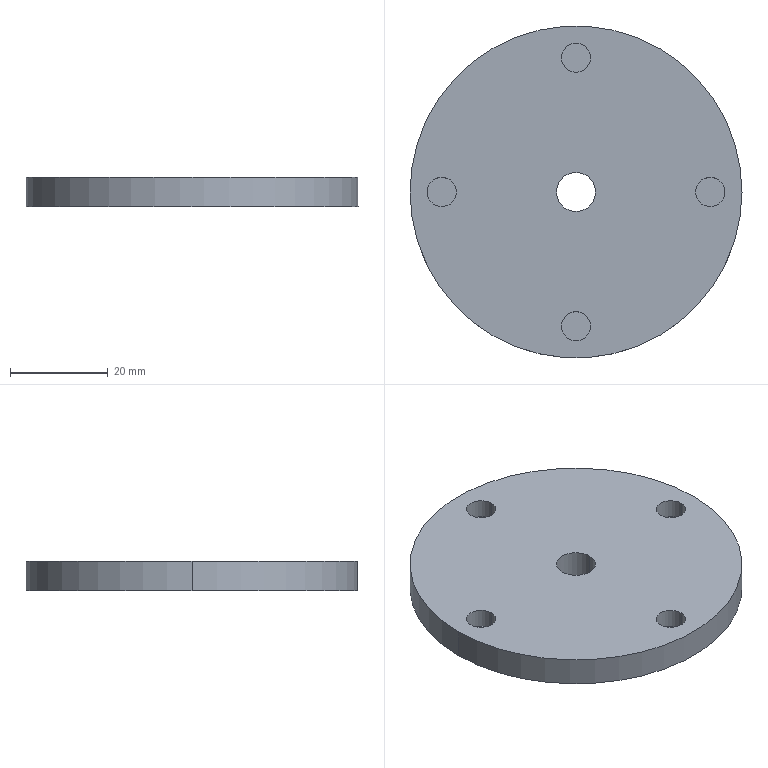Part | SolidWorks | features ICE 2, Extrusion 1 | 1 solid | 18 faces | box 68 x 68 x 6 mm | volume 21036 mm3 | cylinder 12 | plane 6 | commonest cylinder face diameters 6 x8 8 x2 68 x2
STEP:
#1=CARTESIAN_POINT('',(-4.,0.,0.));
#2=VERTEX_POINT('',#1);
#3=CARTESIAN_POINT('',(4.,0.,0.));
#4=VERTEX_POINT('',#3);
#5=CARTESIAN_POINT('',(0.,0.,0.));
#6=DIRECTION('',(0.,0.,1.));
#7=DIRECTION('',(1.,0.,0.));
#8=AXIS2_PLACEMENT_3D('',#5,#6,#7);
#9=CIRCLE('',#8,4.);
#10=EDGE_CURVE('',#2,#4,#9,.T.);
#11=ORIENTED_EDGE('',*,*,#10,.F.);
#12=CARTESIAN_POINT('',(-4.,0.,6.));
#13=VERTEX_POINT('',#12);
#14=CARTESIAN_POINT('',(-4.,0.,0.));
#15=DIRECTION('',(0.,0.,1.));
#16=VECTOR('',#15,1000.);
#17=LINE('',#14,#16);
#18=EDGE_CURVE('',#2,#13,#17,.T.);
#19=ORIENTED_EDGE('',*,*,#18,.T.);
#20=CARTESIAN_POINT('',(4.,0.,6.));
#21=VERTEX_POINT('',#20);
#22=CARTESIAN_POINT('',(0.,0.,6.));
#23=DIRECTION('',(0.,0.,1.));
#24=DIRECTION('',(1.,0.,0.));
#25=AXIS2_PLACEMENT_3D('',#22,#23,#24);
#26=CIRCLE('',#25,4.);
#27=EDGE_CURVE('',#13,#21,#26,.T.);
#28=ORIENTED_EDGE('',*,*,#27,.T.);
#29=CARTESIAN_POINT('',(4.,0.,0.));
#30=DIRECTION('',(0.,0.,1.));
#31=VECTOR('',#30,1000.);
#32=LINE('',#29,#31);
#33=EDGE_CURVE('',#4,#21,#32,.T.);
#34=ORIENTED_EDGE('',*,*,#33,.F.);
#35=EDGE_LOOP('',(#11,#19,#28,#34));
#36=FACE_OUTER_BOUND('',#35,.T.);
#37=CARTESIAN_POINT('',(0.,0.,0.));
#38=DIRECTION('',(0.,0.,1.));
#39=DIRECTION('',(1.,0.,0.));
#40=AXIS2_PLACEMENT_3D('',#37,#38,#39);
#41=CYLINDRICAL_SURFACE('',#40,4.);
#42=ADVANCED_FACE('',(#36),#41,.F.);
#43=CARTESIAN_POINT('',(-3.,27.5,2.));
#44=VERTEX_POINT('',#43);
#45=CARTESIAN_POINT('',(3.,27.5,2.));
#46=VERTEX_POINT('',#45);
#47=CARTESIAN_POINT('',(0.,27.5,2.));
#48=DIRECTION('',(0.,0.,1.));
#49=DIRECTION('',(1.,0.,0.));
#50=AXIS2_PLACEMENT_3D('',#47,#48,#49);
#51=CIRCLE('',#50,3.);
#52=EDGE_CURVE('',#44,#46,#51,.T.);
#53=ORIENTED_EDGE('',*,*,#52,.F.);
#54=CARTESIAN_POINT('',(-3.,27.5,6.));
#55=VERTEX_POINT('',#54);
#56=CARTESIAN_POINT('',(-3.,27.5,2.));
#57=DIRECTION('',(0.,0.,1.));
#58=VECTOR('',#57,1000.);
#59=LINE('',#56,#58);
#60=EDGE_CURVE('',#44,#55,#59,.T.);
#61=ORIENTED_EDGE('',*,*,#60,.T.);
#62=CARTESIAN_POINT('',(3.,27.5,6.));
#63=VERTEX_POINT('',#62);
#64=CARTESIAN_POINT('',(0.,27.5,6.));
#65=DIRECTION('',(0.,0.,1.));
#66=DIRECTION('',(1.,0.,0.));
#67=AXIS2_PLACEMENT_3D('',#64,#65,#66);
#68=CIRCLE('',#67,3.);
#69=EDGE_CURVE('',#55,#63,#68,.T.);
#70=ORIENTED_EDGE('',*,*,#69,.T.);
#71=CARTESIAN_POINT('',(3.,27.5,2.));
#72=DIRECTION('',(0.,0.,1.));
#73=VECTOR('',#72,1000.);
#74=LINE('',#71,#73);
#75=EDGE_CURVE('',#46,#63,#74,.T.);
#76=ORIENTED_EDGE('',*,*,#75,.F.);
#77=EDGE_LOOP('',(#53,#61,#70,#76));
#78=FACE_OUTER_BOUND('',#77,.T.);
#79=CARTESIAN_POINT('',(0.,27.5,2.));
#80=DIRECTION('',(0.,0.,1.));
#81=DIRECTION('',(1.,0.,0.));
#82=AXIS2_PLACEMENT_3D('',#79,#80,#81);
#83=CYLINDRICAL_SURFACE('',#82,3.);
#84=ADVANCED_FACE('',(#78),#83,.F.);
#85=CARTESIAN_POINT('',(24.5,0.,2.));
#86=VERTEX_POINT('',#85);
#87=CARTESIAN_POINT('',(30.5,0.,2.));
#88=VERTEX_POINT('',#87);
#89=CARTESIAN_POINT('',(27.5,0.,2.));
#90=DIRECTION('',(0.,0.,1.));
#91=DIRECTION('',(1.,0.,0.));
#92=AXIS2_PLACEMENT_3D('',#89,#90,#91);
#93=CIRCLE('',#92,3.);
#94=EDGE_CURVE('',#86,#88,#93,.T.);
#95=ORIENTED_EDGE('',*,*,#94,.F.);
#96=CARTESIAN_POINT('',(24.5,0.,6.));
#97=VERTEX_POINT('',#96);
#98=CARTESIAN_POINT('',(24.5,0.,2.));
#99=DIRECTION('',(0.,0.,1.));
#100=VECTOR('',#99,1000.);
#101=LINE('',#98,#100);
#102=EDGE_CURVE('',#86,#97,#101,.T.);
#103=ORIENTED_EDGE('',*,*,#102,.T.);
#104=CARTESIAN_POINT('',(30.5,0.,6.));
#105=VERTEX_POINT('',#104);
#106=CARTESIAN_POINT('',(27.5,0.,6.));
#107=DIRECTION('',(0.,0.,1.));
#108=DIRECTION('',(1.,0.,0.));
#109=AXIS2_PLACEMENT_3D('',#106,#107,#108);
#110=CIRCLE('',#109,3.);
#111=EDGE_CURVE('',#97,#105,#110,.T.);
#112=ORIENTED_EDGE('',*,*,#111,.T.);
#113=CARTESIAN_POINT('',(30.5,0.,2.));
#114=DIRECTION('',(0.,0.,1.));
#115=VECTOR('',#114,1000.);
#116=LINE('',#113,#115);
#117=EDGE_CURVE('',#88,#105,#116,.T.);
#118=ORIENTED_EDGE('',*,*,#117,.F.);
#119=EDGE_LOOP('',(#95,#103,#112,#118));
#120=FACE_OUTER_BOUND('',#119,.T.);
#121=CARTESIAN_POINT('',(27.5,0.,2.));
#122=DIRECTION('',(0.,0.,1.));
#123=DIRECTION('',(1.,0.,0.));
#124=AXIS2_PLACEMENT_3D('',#121,#122,#123);
#125=CYLINDRICAL_SURFACE('',#124,3.);
#126=ADVANCED_FACE('',(#120),#125,.F.);
#127=CARTESIAN_POINT('',(-3.,-27.5,2.));
#128=VERTEX_POINT('',#127);
#129=CARTESIAN_POINT('',(3.,-27.5,2.));
#130=VERTEX_POINT('',#129);
#131=CARTESIAN_POINT('',(0.,-27.5,2.));
#132=DIRECTION('',(0.,0.,1.));
#133=DIRECTION('',(1.,0.,0.));
#134=AXIS2_PLACEMENT_3D('',#131,#132,#133);
#135=CIRCLE('',#134,3.);
#136=EDGE_CURVE('',#128,#130,#135,.T.);
#137=ORIENTED_EDGE('',*,*,#136,.F.);
#138=CARTESIAN_POINT('',(-3.,-27.5,6.));
#139=VERTEX_POINT('',#138);
#140=CARTESIAN_POINT('',(-3.,-27.5,2.));
#141=DIRECTION('',(0.,0.,1.));
#142=VECTOR('',#141,1000.);
#143=LINE('',#140,#142);
#144=EDGE_CURVE('',#128,#139,#143,.T.);
#145=ORIENTED_EDGE('',*,*,#144,.T.);
#146=CARTESIAN_POINT('',(3.,-27.5,6.));
#147=VERTEX_POINT('',#146);
#148=CARTESIAN_POINT('',(0.,-27.5,6.));
#149=DIRECTION('',(0.,0.,1.));
#150=DIRECTION('',(1.,0.,0.));
#151=AXIS2_PLACEMENT_3D('',#148,#149,#150);
#152=CIRCLE('',#151,3.);
#153=EDGE_CURVE('',#139,#147,#152,.T.);
#154=ORIENTED_EDGE('',*,*,#153,.T.);
#155=CARTESIAN_POINT('',(3.,-27.5,2.));
#156=DIRECTION('',(0.,0.,1.));
#157=VECTOR('',#156,1000.);
#158=LINE('',#155,#157);
#159=EDGE_CURVE('',#130,#147,#158,.T.);
#160=ORIENTED_EDGE('',*,*,#159,.F.);
#161=EDGE_LOOP('',(#137,#145,#154,#160));
#162=FACE_OUTER_BOUND('',#161,.T.);
#163=CARTESIAN_POINT('',(0.,-27.5,2.));
#164=DIRECTION('',(0.,0.,1.));
#165=DIRECTION('',(1.,0.,0.));
#166=AXIS2_PLACEMENT_3D('',#163,#164,#165);
#167=CYLINDRICAL_SURFACE('',#166,3.);
#168=ADVANCED_FACE('',(#162),#167,.F.);
#169=CARTESIAN_POINT('',(-30.5,0.,2.));
#170=VERTEX_POINT('',#169);
#171=CARTESIAN_POINT('',(-24.5,0.,2.));
#172=VERTEX_POINT('',#171);
#173=CARTESIAN_POINT('',(-27.5,0.,2.));
#174=DIRECTION('',(0.,0.,1.));
#175=DIRECTION('',(1.,0.,0.));
#176=AXIS2_PLACEMENT_3D('',#173,#174,#175);
#177=CIRCLE('',#176,3.);
#178=EDGE_CURVE('',#170,#172,#177,.T.);
#179=ORIENTED_EDGE('',*,*,#178,.F.);
#180=CARTESIAN_POINT('',(-30.5,0.,6.));
#181=VERTEX_POINT('',#180);
#182=CARTESIAN_POINT('',(-30.5,0.,2.));
#183=DIRECTION('',(0.,0.,1.));
#184=VECTOR('',#183,1000.);
#185=LINE('',#182,#184);
#186=EDGE_CURVE('',#170,#181,#185,.T.);
#187=ORIENTED_EDGE('',*,*,#186,.T.);
#188=CARTESIAN_POINT('',(-24.5,0.,6.));
#189=VERTEX_POINT('',#188);
#190=CARTESIAN_POINT('',(-27.5,0.,6.));
#191=DIRECTION('',(0.,0.,1.));
#192=DIRECTION('',(1.,0.,0.));
#193=AXIS2_PLACEMENT_3D('',#190,#191,#192);
#194=CIRCLE('',#193,3.);
#195=EDGE_CURVE('',#181,#189,#194,.T.);
#196=ORIENTED_EDGE('',*,*,#195,.T.);
#197=CARTESIAN_POINT('',(-24.5,0.,2.));
#198=DIRECTION('',(0.,0.,1.));
#199=VECTOR('',#198,1000.);
#200=LINE('',#197,#199);
#201=EDGE_CURVE('',#172,#189,#200,.T.);
#202=ORIENTED_EDGE('',*,*,#201,.F.);
#203=EDGE_LOOP('',(#179,#187,#196,#202));
#204=FACE_OUTER_BOUND('',#203,.T.);
#205=CARTESIAN_POINT('',(-27.5,0.,2.));
#206=DIRECTION('',(0.,0.,1.));
#207=DIRECTION('',(1.,0.,0.));
#208=AXIS2_PLACEMENT_3D('',#205,#206,#207);
#209=CYLINDRICAL_SURFACE('',#208,3.);
#210=ADVANCED_FACE('',(#204),#209,.F.);
#211=CARTESIAN_POINT('',(34.,0.,6.));
#212=VERTEX_POINT('',#211);
#213=CARTESIAN_POINT('',(-34.,0.,6.));
#214=VERTEX_POINT('',#213);
#215=CARTESIAN_POINT('',(0.,0.,6.));
#216=DIRECTION('',(0.,0.,1.));
#217=DIRECTION('',(1.,0.,0.));
#218=AXIS2_PLACEMENT_3D('',#215,#216,#217);
#219=CIRCLE('',#218,34.);
#220=EDGE_CURVE('',#212,#214,#219,.T.);
#221=ORIENTED_EDGE('',*,*,#220,.F.);
#222=CARTESIAN_POINT('',(34.,0.,0.));
#223=VERTEX_POINT('',#222);
#224=CARTESIAN_POINT('',(34.,0.,6.));
#225=DIRECTION('',(0.,0.,-1.));
#226=VECTOR('',#225,1000.);
#227=LINE('',#224,#226);
#228=EDGE_CURVE('',#212,#223,#227,.T.);
#229=ORIENTED_EDGE('',*,*,#228,.T.);
#230=CARTESIAN_POINT('',(-34.,0.,0.));
#231=VERTEX_POINT('',#230);
#232=CARTESIAN_POINT('',(0.,0.,0.));
#233=DIRECTION('',(0.,0.,1.));
#234=DIRECTION('',(1.,0.,0.));
#235=AXIS2_PLACEMENT_3D('',#232,#233,#234);
#236=CIRCLE('',#235,34.);
#237=EDGE_CURVE('',#223,#231,#236,.T.);
#238=ORIENTED_EDGE('',*,*,#237,.T.);
#239=CARTESIAN_POINT('',(-34.,0.,6.));
#240=DIRECTION('',(0.,0.,-1.));
#241=VECTOR('',#240,1000.);
#242=LINE('',#239,#241);
#243=EDGE_CURVE('',#214,#231,#242,.T.);
#244=ORIENTED_EDGE('',*,*,#243,.F.);
#245=EDGE_LOOP('',(#221,#229,#238,#244));
#246=FACE_OUTER_BOUND('',#245,.T.);
#247=CARTESIAN_POINT('',(0.,0.,6.));
#248=DIRECTION('',(0.,0.,-1.));
#249=DIRECTION('',(-1.,0.,0.));
#250=AXIS2_PLACEMENT_3D('',#247,#248,#249);
#251=CYLINDRICAL_SURFACE('',#250,34.);
#252=ADVANCED_FACE('',(#246),#251,.T.);
#253=ORIENTED_EDGE('',*,*,#228,.F.);
#254=CARTESIAN_POINT('',(0.,0.,6.));
#255=DIRECTION('',(0.,0.,1.));
#256=DIRECTION('',(1.,0.,0.));
#257=AXIS2_PLACEMENT_3D('',#254,#255,#256);
#258=CIRCLE('',#257,34.);
#259=EDGE_CURVE('',#214,#212,#258,.T.);
#260=ORIENTED_EDGE('',*,*,#259,.F.);
#261=ORIENTED_EDGE('',*,*,#243,.T.);
#262=CARTESIAN_POINT('',(0.,0.,0.));
#263=DIRECTION('',(0.,0.,1.));
#264=DIRECTION('',(1.,0.,0.));
#265=AXIS2_PLACEMENT_3D('',#262,#263,#264);
#266=CIRCLE('',#265,34.);
#267=EDGE_CURVE('',#231,#223,#266,.T.);
#268=ORIENTED_EDGE('',*,*,#267,.T.);
#269=EDGE_LOOP('',(#253,#260,#261,#268));
#270=FACE_OUTER_BOUND('',#269,.T.);
#271=CARTESIAN_POINT('',(0.,0.,6.));
#272=DIRECTION('',(0.,0.,-1.));
#273=DIRECTION('',(-1.,0.,0.));
#274=AXIS2_PLACEMENT_3D('',#271,#272,#273);
#275=CYLINDRICAL_SURFACE('',#274,34.);
#276=ADVANCED_FACE('',(#270),#275,.T.);
#277=CARTESIAN_POINT('',(0.,0.,6.));
#278=DIRECTION('',(0.,0.,1.));
#279=DIRECTION('',(1.,0.,0.));
#280=AXIS2_PLACEMENT_3D('',#277,#278,#279);
#281=CIRCLE('',#280,4.);
#282=EDGE_CURVE('',#21,#13,#281,.T.);
#283=ORIENTED_EDGE('',*,*,#282,.F.);
#284=ORIENTED_EDGE('',*,*,#27,.F.);
#285=EDGE_LOOP('',(#283,#284));
#286=FACE_BOUND('',#285,.T.);
#287=CARTESIAN_POINT('',(0.,27.5,6.));
#288=DIRECTION('',(0.,0.,1.));
#289=DIRECTION('',(1.,0.,0.));
#290=AXIS2_PLACEMENT_3D('',#287,#288,#289);
#291=CIRCLE('',#290,3.);
#292=EDGE_CURVE('',#63,#55,#291,.T.);
#293=ORIENTED_EDGE('',*,*,#292,.F.);
#294=ORIENTED_EDGE('',*,*,#69,.F.);
#295=EDGE_LOOP('',(#293,#294));
#296=FACE_BOUND('',#295,.T.);
#297=CARTESIAN_POINT('',(27.5,0.,6.));
#298=DIRECTION('',(0.,0.,1.));
#299=DIRECTION('',(1.,0.,0.));
#300=AXIS2_PLACEMENT_3D('',#297,#298,#299);
#301=CIRCLE('',#300,3.);
#302=EDGE_CURVE('',#105,#97,#301,.T.);
#303=ORIENTED_EDGE('',*,*,#302,.F.);
#304=ORIENTED_EDGE('',*,*,#111,.F.);
#305=EDGE_LOOP('',(#303,#304));
#306=FACE_BOUND('',#305,.T.);
#307=CARTESIAN_POINT('',(0.,-27.5,6.));
#308=DIRECTION('',(0.,0.,1.));
#309=DIRECTION('',(1.,0.,0.));
#310=AXIS2_PLACEMENT_3D('',#307,#308,#309);
#311=CIRCLE('',#310,3.);
#312=EDGE_CURVE('',#147,#139,#311,.T.);
#313=ORIENTED_EDGE('',*,*,#312,.F.);
#314=ORIENTED_EDGE('',*,*,#153,.F.);
#315=EDGE_LOOP('',(#313,#314));
#316=FACE_BOUND('',#315,.T.);
#317=CARTESIAN_POINT('',(-27.5,0.,6.));
#318=DIRECTION('',(0.,0.,1.));
#319=DIRECTION('',(1.,0.,0.));
#320=AXIS2_PLACEMENT_3D('',#317,#318,#319);
#321=CIRCLE('',#320,3.);
#322=EDGE_CURVE('',#189,#181,#321,.T.);
#323=ORIENTED_EDGE('',*,*,#322,.F.);
#324=ORIENTED_EDGE('',*,*,#195,.F.);
#325=EDGE_LOOP('',(#323,#324));
#326=FACE_BOUND('',#325,.T.);
#327=ORIENTED_EDGE('',*,*,#259,.T.);
#328=ORIENTED_EDGE('',*,*,#220,.T.);
#329=EDGE_LOOP('',(#327,#328));
#330=FACE_OUTER_BOUND('',#329,.T.);
#331=CARTESIAN_POINT('',(0.,0.,6.));
#332=DIRECTION('',(0.,0.,1.));
#333=DIRECTION('',(1.,0.,0.));
#334=AXIS2_PLACEMENT_3D('',#331,#332,#333);
#335=PLANE('',#334);
#336=ADVANCED_FACE('',(#286,#296,#306,#316,#326,#330),#335,.T.);
#337=CARTESIAN_POINT('',(0.,0.,0.));
#338=DIRECTION('',(0.,0.,1.));
#339=DIRECTION('',(1.,0.,0.));
#340=AXIS2_PLACEMENT_3D('',#337,#338,#339);
#341=CIRCLE('',#340,4.);
#342=EDGE_CURVE('',#4,#2,#341,.T.);
#343=ORIENTED_EDGE('',*,*,#342,.T.);
#344=ORIENTED_EDGE('',*,*,#10,.T.);
#345=EDGE_LOOP('',(#343,#344));
#346=FACE_BOUND('',#345,.T.);
#347=ORIENTED_EDGE('',*,*,#267,.F.);
#348=ORIENTED_EDGE('',*,*,#237,.F.);
#349=EDGE_LOOP('',(#347,#348));
#350=FACE_OUTER_BOUND('',#349,.T.);
#351=CARTESIAN_POINT('',(0.,0.,0.));
#352=DIRECTION('',(0.,0.,1.));
#353=DIRECTION('',(1.,0.,0.));
#354=AXIS2_PLACEMENT_3D('',#351,#352,#353);
#355=PLANE('',#354);
#356=ADVANCED_FACE('',(#346,#350),#355,.F.);
#357=ORIENTED_EDGE('',*,*,#186,.F.);
#358=CARTESIAN_POINT('',(-27.5,0.,2.));
#359=DIRECTION('',(0.,0.,1.));
#360=DIRECTION('',(1.,0.,0.));
#361=AXIS2_PLACEMENT_3D('',#358,#359,#360);
#362=CIRCLE('',#361,3.);
#363=EDGE_CURVE('',#172,#170,#362,.T.);
#364=ORIENTED_EDGE('',*,*,#363,.F.);
#365=ORIENTED_EDGE('',*,*,#201,.T.);
#366=ORIENTED_EDGE('',*,*,#322,.T.);
#367=EDGE_LOOP('',(#357,#364,#365,#366));
#368=FACE_OUTER_BOUND('',#367,.T.);
#369=CARTESIAN_POINT('',(-27.5,0.,2.));
#370=DIRECTION('',(0.,0.,1.));
#371=DIRECTION('',(1.,0.,0.));
#372=AXIS2_PLACEMENT_3D('',#369,#370,#371);
#373=CYLINDRICAL_SURFACE('',#372,3.);
#374=ADVANCED_FACE('',(#368),#373,.F.);
#375=ORIENTED_EDGE('',*,*,#363,.T.);
#376=ORIENTED_EDGE('',*,*,#178,.T.);
#377=EDGE_LOOP('',(#375,#376));
#378=FACE_OUTER_BOUND('',#377,.T.);
#379=CARTESIAN_POINT('',(-27.5,0.,2.));
#380=DIRECTION('',(0.,0.,1.));
#381=DIRECTION('',(1.,0.,0.));
#382=AXIS2_PLACEMENT_3D('',#379,#380,#381);
#383=PLANE('',#382);
#384=ADVANCED_FACE('',(#378),#383,.T.);
#385=ORIENTED_EDGE('',*,*,#144,.F.);
#386=CARTESIAN_POINT('',(0.,-27.5,2.));
#387=DIRECTION('',(0.,0.,1.));
#388=DIRECTION('',(1.,0.,0.));
#389=AXIS2_PLACEMENT_3D('',#386,#387,#388);
#390=CIRCLE('',#389,3.);
#391=EDGE_CURVE('',#130,#128,#390,.T.);
#392=ORIENTED_EDGE('',*,*,#391,.F.);
#393=ORIENTED_EDGE('',*,*,#159,.T.);
#394=ORIENTED_EDGE('',*,*,#312,.T.);
#395=EDGE_LOOP('',(#385,#392,#393,#394));
#396=FACE_OUTER_BOUND('',#395,.T.);
#397=CARTESIAN_POINT('',(0.,-27.5,2.));
#398=DIRECTION('',(0.,0.,1.));
#399=DIRECTION('',(1.,0.,0.));
#400=AXIS2_PLACEMENT_3D('',#397,#398,#399);
#401=CYLINDRICAL_SURFACE('',#400,3.);
#402=ADVANCED_FACE('',(#396),#401,.F.);
#403=ORIENTED_EDGE('',*,*,#391,.T.);
#404=ORIENTED_EDGE('',*,*,#136,.T.);
#405=EDGE_LOOP('',(#403,#404));
#406=FACE_OUTER_BOUND('',#405,.T.);
#407=CARTESIAN_POINT('',(0.,-27.5,2.));
#408=DIRECTION('',(0.,0.,1.));
#409=DIRECTION('',(1.,0.,0.));
#410=AXIS2_PLACEMENT_3D('',#407,#408,#409);
#411=PLANE('',#410);
#412=ADVANCED_FACE('',(#406),#411,.T.);
#413=ORIENTED_EDGE('',*,*,#102,.F.);
#414=CARTESIAN_POINT('',(27.5,0.,2.));
#415=DIRECTION('',(0.,0.,1.));
#416=DIRECTION('',(1.,0.,0.));
#417=AXIS2_PLACEMENT_3D('',#414,#415,#416);
#418=CIRCLE('',#417,3.);
#419=EDGE_CURVE('',#88,#86,#418,.T.);
#420=ORIENTED_EDGE('',*,*,#419,.F.);
#421=ORIENTED_EDGE('',*,*,#117,.T.);
#422=ORIENTED_EDGE('',*,*,#302,.T.);
#423=EDGE_LOOP('',(#413,#420,#421,#422));
#424=FACE_OUTER_BOUND('',#423,.T.);
#425=CARTESIAN_POINT('',(27.5,0.,2.));
#426=DIRECTION('',(0.,0.,1.));
#427=DIRECTION('',(1.,0.,0.));
#428=AXIS2_PLACEMENT_3D('',#425,#426,#427);
#429=CYLINDRICAL_SURFACE('',#428,3.);
#430=ADVANCED_FACE('',(#424),#429,.F.);
#431=ORIENTED_EDGE('',*,*,#419,.T.);
#432=ORIENTED_EDGE('',*,*,#94,.T.);
#433=EDGE_LOOP('',(#431,#432));
#434=FACE_OUTER_BOUND('',#433,.T.);
#435=CARTESIAN_POINT('',(27.5,0.,2.));
#436=DIRECTION('',(0.,0.,1.));
#437=DIRECTION('',(1.,0.,0.));
#438=AXIS2_PLACEMENT_3D('',#435,#436,#437);
#439=PLANE('',#438);
#440=ADVANCED_FACE('',(#434),#439,.T.);
#441=ORIENTED_EDGE('',*,*,#60,.F.);
#442=CARTESIAN_POINT('',(0.,27.5,2.));
#443=DIRECTION('',(0.,0.,1.));
#444=DIRECTION('',(1.,0.,0.));
#445=AXIS2_PLACEMENT_3D('',#442,#443,#444);
#446=CIRCLE('',#445,3.);
#447=EDGE_CURVE('',#46,#44,#446,.T.);
#448=ORIENTED_EDGE('',*,*,#447,.F.);
#449=ORIENTED_EDGE('',*,*,#75,.T.);
#450=ORIENTED_EDGE('',*,*,#292,.T.);
#451=EDGE_LOOP('',(#441,#448,#449,#450));
#452=FACE_OUTER_BOUND('',#451,.T.);
#453=CARTESIAN_POINT('',(0.,27.5,2.));
#454=DIRECTION('',(0.,0.,1.));
#455=DIRECTION('',(1.,0.,0.));
#456=AXIS2_PLACEMENT_3D('',#453,#454,#455);
#457=CYLINDRICAL_SURFACE('',#456,3.);
#458=ADVANCED_FACE('',(#452),#457,.F.);
#459=ORIENTED_EDGE('',*,*,#447,.T.);
#460=ORIENTED_EDGE('',*,*,#52,.T.);
#461=EDGE_LOOP('',(#459,#460));
#462=FACE_OUTER_BOUND('',#461,.T.);
#463=CARTESIAN_POINT('',(0.,27.5,2.));
#464=DIRECTION('',(0.,0.,1.));
#465=DIRECTION('',(1.,0.,0.));
#466=AXIS2_PLACEMENT_3D('',#463,#464,#465);
#467=PLANE('',#466);
#468=ADVANCED_FACE('',(#462),#467,.T.);
#469=ORIENTED_EDGE('',*,*,#18,.F.);
#470=ORIENTED_EDGE('',*,*,#342,.F.);
#471=ORIENTED_EDGE('',*,*,#33,.T.);
#472=ORIENTED_EDGE('',*,*,#282,.T.);
#473=EDGE_LOOP('',(#469,#470,#471,#472));
#474=FACE_OUTER_BOUND('',#473,.T.);
#475=CARTESIAN_POINT('',(0.,0.,0.));
#476=DIRECTION('',(0.,0.,1.));
#477=DIRECTION('',(1.,0.,0.));
#478=AXIS2_PLACEMENT_3D('',#475,#476,#477);
#479=CYLINDRICAL_SURFACE('',#478,4.);
#480=ADVANCED_FACE('',(#474),#479,.F.);
#481=CLOSED_SHELL('',(#42,#84,#126,#168,#210,#252,#276,#336,#356,#374,#384,#402,#412,#430,#440,#458,#468,#480));
#482=MANIFOLD_SOLID_BREP('',#481);
#483=CARTESIAN_POINT('',(0.,0.,0.));
#484=DIRECTION('',(0.,0.,1.));
#485=DIRECTION('',(1.,0.,0.));
#486=AXIS2_PLACEMENT_3D('',#483,#484,#485);
#487=(LENGTH_UNIT()NAMED_UNIT(*)SI_UNIT(.MILLI.,.METRE.));
#488=UNCERTAINTY_MEASURE_WITH_UNIT(LENGTH_MEASURE(0.00001),#487,'','');
#489=(NAMED_UNIT(*)PLANE_ANGLE_UNIT()SI_UNIT($,.RADIAN.));
#490=(NAMED_UNIT(*)SI_UNIT($,.STERADIAN.)SOLID_ANGLE_UNIT());
#491=(GEOMETRIC_REPRESENTATION_CONTEXT(3)GLOBAL_UNCERTAINTY_ASSIGNED_CONTEXT((#488))GLOBAL_UNIT_ASSIGNED_CONTEXT((#487,#489,#490))REPRESENTATION_CONTEXT('',''));
#492=ADVANCED_BREP_SHAPE_REPRESENTATION('',(#482,#486),#491);